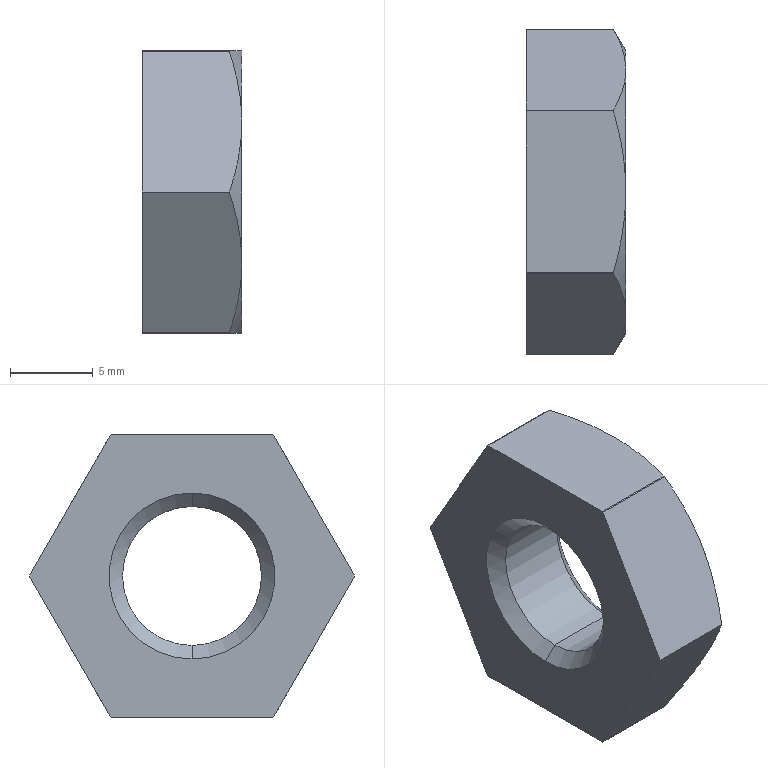Part | STEP file | 0217_Z_ANBNS10-80-2 | 1 solid | 24 faces | box 6 x 19.6 x 17 mm | volume 1146 mm3 | cone 10 | plane 8 | cylinder 6 | commonest cylinder face diameters 19.6 x4 8.376 x2